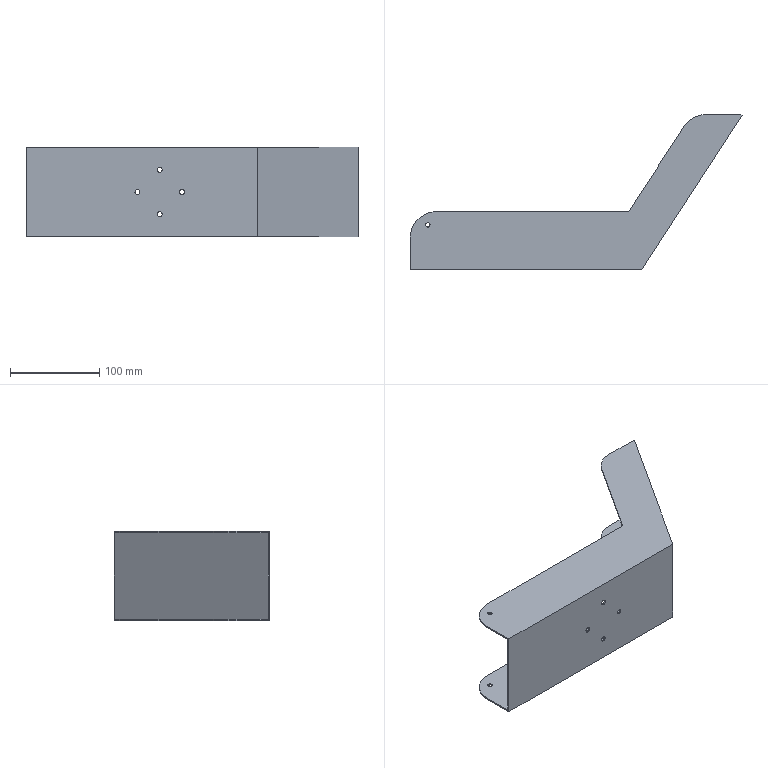Part | NX | 1 solid | 32 faces | box 372.47 x 174.005 x 100 mm | volume 140238 mm3 | plane 16 | cylinder 16 | commonest cylinder face diameters 5.5 x8 5 x4 60 x4
STEP:
#1=CARTESIAN_POINT('',(-165.999,174.005,50.));
#2=VERTEX_POINT('',#1);
#3=CARTESIAN_POINT('',(-127.288,174.005,50.));
#4=VERTEX_POINT('',#3);
#5=CARTESIAN_POINT('',(0.,174.005,50.));
#6=DIRECTION('',(1.,0.,0.));
#7=VECTOR('',#6,1000.);
#8=LINE('',#5,#7);
#9=EDGE_CURVE('',#2,#4,#8,.T.);
#10=ORIENTED_EDGE('',*,*,#9,.F.);
#11=CARTESIAN_POINT('',(-191.16,160.345,50.));
#12=VERTEX_POINT('',#11);
#13=CARTESIAN_POINT('',(-165.999,144.005,50.));
#14=DIRECTION('',(0.,0.,-1.));
#15=DIRECTION('',(-1.,0.,0.));
#16=AXIS2_PLACEMENT_3D('',#13,#14,#15);
#17=CIRCLE('',#16,30.);
#18=EDGE_CURVE('',#12,#2,#17,.T.);
#19=ORIENTED_EDGE('',*,*,#18,.F.);
#20=CARTESIAN_POINT('',(-253.077,65.,50.));
#21=VERTEX_POINT('',#20);
#22=CARTESIAN_POINT('',(-295.289,0.,50.));
#23=DIRECTION('',(0.5446,0.8387,0.));
#24=VECTOR('',#23,1000.);
#25=LINE('',#22,#24);
#26=EDGE_CURVE('',#21,#12,#25,.T.);
#27=ORIENTED_EDGE('',*,*,#26,.F.);
#28=CARTESIAN_POINT('',(-468.5,65.,50.));
#29=VERTEX_POINT('',#28);
#30=CARTESIAN_POINT('',(0.,65.,50.));
#31=DIRECTION('',(1.,0.,0.));
#32=VECTOR('',#31,1000.);
#33=LINE('',#30,#32);
#34=EDGE_CURVE('',#29,#21,#33,.T.);
#35=ORIENTED_EDGE('',*,*,#34,.F.);
#36=CARTESIAN_POINT('',(-498.5,35.,50.));
#37=VERTEX_POINT('',#36);
#38=CARTESIAN_POINT('',(-468.5,35.,50.));
#39=DIRECTION('',(0.,0.,1.));
#40=DIRECTION('',(1.,0.,0.));
#41=AXIS2_PLACEMENT_3D('',#38,#39,#40);
#42=CIRCLE('',#41,30.);
#43=EDGE_CURVE('',#29,#37,#42,.T.);
#44=ORIENTED_EDGE('',*,*,#43,.T.);
#45=CARTESIAN_POINT('',(-498.5,0.,50.));
#46=VERTEX_POINT('',#45);
#47=CARTESIAN_POINT('',(-498.5,0.,50.));
#48=DIRECTION('',(0.,-1.,0.));
#49=VECTOR('',#48,1000.);
#50=LINE('',#47,#49);
#51=EDGE_CURVE('',#37,#46,#50,.T.);
#52=ORIENTED_EDGE('',*,*,#51,.T.);
#53=CARTESIAN_POINT('',(-238.5,0.,50.));
#54=VERTEX_POINT('',#53);
#55=CARTESIAN_POINT('',(0.,0.,50.));
#56=DIRECTION('',(-1.,0.,0.));
#57=VECTOR('',#56,1000.);
#58=LINE('',#55,#57);
#59=EDGE_CURVE('',#54,#46,#58,.T.);
#60=ORIENTED_EDGE('',*,*,#59,.F.);
#61=CARTESIAN_POINT('',(-126.03,173.189,50.));
#62=VERTEX_POINT('',#61);
#63=CARTESIAN_POINT('',(-238.5,0.,50.));
#64=DIRECTION('',(-0.5446,-0.8387,0.));
#65=VECTOR('',#64,1000.);
#66=LINE('',#63,#65);
#67=EDGE_CURVE('',#62,#54,#66,.T.);
#68=ORIENTED_EDGE('',*,*,#67,.F.);
#69=CARTESIAN_POINT('',(0.,91.344,50.));
#70=DIRECTION('',(0.8387,-0.5446,0.));
#71=VECTOR('',#70,1000.);
#72=LINE('',#69,#71);
#73=EDGE_CURVE('',#4,#62,#72,.T.);
#74=ORIENTED_EDGE('',*,*,#73,.F.);
#75=EDGE_LOOP('',(#10,#19,#27,#35,#44,#52,#60,#68,#74));
#76=FACE_BOUND('',#75,.T.);
#77=CARTESIAN_POINT('',(-481.,50.,50.));
#78=VERTEX_POINT('',#77);
#79=CARTESIAN_POINT('',(-476.,50.,50.));
#80=VERTEX_POINT('',#79);
#81=CARTESIAN_POINT('',(-478.5,50.,50.));
#82=DIRECTION('',(0.,0.,1.));
#83=DIRECTION('',(1.,0.,0.));
#84=AXIS2_PLACEMENT_3D('',#81,#82,#83);
#85=CIRCLE('',#84,2.5);
#86=EDGE_CURVE('',#78,#80,#85,.T.);
#87=ORIENTED_EDGE('',*,*,#86,.F.);
#88=CARTESIAN_POINT('',(-478.5,50.,50.));
#89=DIRECTION('',(0.,0.,1.));
#90=DIRECTION('',(1.,0.,0.));
#91=AXIS2_PLACEMENT_3D('',#88,#89,#90);
#92=CIRCLE('',#91,2.5);
#93=EDGE_CURVE('',#80,#78,#92,.T.);
#94=ORIENTED_EDGE('',*,*,#93,.F.);
#95=EDGE_LOOP('',(#87,#94));
#96=FACE_BOUND('',#95,.T.);
#97=CARTESIAN_POINT('',(-221.19,55.831,50.));
#98=DIRECTION('',(0.,0.,1.));
#99=DIRECTION('',(1.,0.,0.));
#100=AXIS2_PLACEMENT_3D('',#97,#98,#99);
#101=PLANE('',#100);
#102=ADVANCED_FACE('',(#76,#96),#101,.T.);
#103=CARTESIAN_POINT('',(-468.5,65.,-48.5));
#104=VERTEX_POINT('',#103);
#105=CARTESIAN_POINT('',(-468.5,65.,-50.));
#106=VERTEX_POINT('',#105);
#107=CARTESIAN_POINT('',(-468.5,65.,0.));
#108=DIRECTION('',(0.,0.,-1.));
#109=VECTOR('',#108,1000.);
#110=LINE('',#107,#109);
#111=EDGE_CURVE('',#104,#106,#110,.T.);
#112=ORIENTED_EDGE('',*,*,#111,.F.);
#113=CARTESIAN_POINT('',(-253.077,65.,-48.5));
#114=VERTEX_POINT('',#113);
#115=CARTESIAN_POINT('',(0.,65.,-48.5));
#116=DIRECTION('',(1.,0.,0.));
#117=VECTOR('',#116,1000.);
#118=LINE('',#115,#117);
#119=EDGE_CURVE('',#104,#114,#118,.T.);
#120=ORIENTED_EDGE('',*,*,#119,.T.);
#121=CARTESIAN_POINT('',(-253.077,65.,-50.));
#122=VERTEX_POINT('',#121);
#123=CARTESIAN_POINT('',(-253.077,65.,0.));
#124=DIRECTION('',(0.,0.,-1.));
#125=VECTOR('',#124,1000.);
#126=LINE('',#123,#125);
#127=EDGE_CURVE('',#114,#122,#126,.T.);
#128=ORIENTED_EDGE('',*,*,#127,.T.);
#129=CARTESIAN_POINT('',(0.,65.,-50.));
#130=DIRECTION('',(1.,0.,0.));
#131=VECTOR('',#130,1000.);
#132=LINE('',#129,#131);
#133=EDGE_CURVE('',#106,#122,#132,.T.);
#134=ORIENTED_EDGE('',*,*,#133,.F.);
#135=EDGE_LOOP('',(#112,#120,#128,#134));
#136=FACE_BOUND('',#135,.T.);
#137=CARTESIAN_POINT('',(-249.25,65.,-59.25));
#138=DIRECTION('',(0.,-1.,0.));
#139=DIRECTION('',(0.,0.,-1.));
#140=AXIS2_PLACEMENT_3D('',#137,#138,#139);
#141=PLANE('',#140);
#142=ADVANCED_FACE('',(#136),#141,.F.);
#143=CARTESIAN_POINT('',(-239.314,1.5,-48.5));
#144=VERTEX_POINT('',#143);
#145=CARTESIAN_POINT('',(-127.288,174.005,-48.5));
#146=VERTEX_POINT('',#145);
#147=CARTESIAN_POINT('',(-240.289,0.,-48.5));
#148=DIRECTION('',(0.5446,0.8387,0.));
#149=VECTOR('',#148,1000.);
#150=LINE('',#147,#149);
#151=EDGE_CURVE('',#144,#146,#150,.T.);
#152=ORIENTED_EDGE('',*,*,#151,.T.);
#153=CARTESIAN_POINT('',(-165.999,174.005,-48.5));
#154=VERTEX_POINT('',#153);
#155=CARTESIAN_POINT('',(0.,174.005,-48.5));
#156=DIRECTION('',(-1.,0.,0.));
#157=VECTOR('',#156,1000.);
#158=LINE('',#155,#157);
#159=EDGE_CURVE('',#146,#154,#158,.T.);
#160=ORIENTED_EDGE('',*,*,#159,.T.);
#161=CARTESIAN_POINT('',(-191.16,160.345,-48.5));
#162=VERTEX_POINT('',#161);
#163=CARTESIAN_POINT('',(-165.999,144.005,-48.5));
#164=DIRECTION('',(0.,0.,1.));
#165=DIRECTION('',(1.,0.,0.));
#166=AXIS2_PLACEMENT_3D('',#163,#164,#165);
#167=CIRCLE('',#166,30.);
#168=EDGE_CURVE('',#154,#162,#167,.T.);
#169=ORIENTED_EDGE('',*,*,#168,.T.);
#170=CARTESIAN_POINT('',(-295.289,0.,-48.5));
#171=DIRECTION('',(-0.5446,-0.8387,0.));
#172=VECTOR('',#171,1000.);
#173=LINE('',#170,#172);
#174=EDGE_CURVE('',#162,#114,#173,.T.);
#175=ORIENTED_EDGE('',*,*,#174,.T.);
#176=ORIENTED_EDGE('',*,*,#119,.F.);
#177=CARTESIAN_POINT('',(-498.5,35.,-48.5));
#178=VERTEX_POINT('',#177);
#179=CARTESIAN_POINT('',(-468.5,35.,-48.5));
#180=DIRECTION('',(0.,0.,-1.));
#181=DIRECTION('',(-1.,0.,0.));
#182=AXIS2_PLACEMENT_3D('',#179,#180,#181);
#183=CIRCLE('',#182,30.);
#184=EDGE_CURVE('',#178,#104,#183,.T.);
#185=ORIENTED_EDGE('',*,*,#184,.F.);
#186=CARTESIAN_POINT('',(-498.5,1.5,-48.5));
#187=VERTEX_POINT('',#186);
#188=CARTESIAN_POINT('',(-498.5,0.,-48.5));
#189=DIRECTION('',(0.,1.,0.));
#190=VECTOR('',#189,1000.);
#191=LINE('',#188,#190);
#192=EDGE_CURVE('',#187,#178,#191,.T.);
#193=ORIENTED_EDGE('',*,*,#192,.F.);
#194=CARTESIAN_POINT('',(0.,1.5,-48.5));
#195=DIRECTION('',(1.,0.,0.));
#196=VECTOR('',#195,1000.);
#197=LINE('',#194,#196);
#198=EDGE_CURVE('',#187,#144,#197,.T.);
#199=ORIENTED_EDGE('',*,*,#198,.T.);
#200=EDGE_LOOP('',(#152,#160,#169,#175,#176,#185,#193,#199));
#201=FACE_BOUND('',#200,.T.);
#202=CARTESIAN_POINT('',(-476.,50.,-48.5));
#203=VERTEX_POINT('',#202);
#204=CARTESIAN_POINT('',(-481.,50.,-48.5));
#205=VERTEX_POINT('',#204);
#206=CARTESIAN_POINT('',(-478.5,50.,-48.5));
#207=DIRECTION('',(0.,0.,1.));
#208=DIRECTION('',(1.,0.,0.));
#209=AXIS2_PLACEMENT_3D('',#206,#207,#208);
#210=CIRCLE('',#209,2.5);
#211=EDGE_CURVE('',#203,#205,#210,.T.);
#212=ORIENTED_EDGE('',*,*,#211,.F.);
#213=CARTESIAN_POINT('',(-478.5,50.,-48.5));
#214=DIRECTION('',(0.,0.,1.));
#215=DIRECTION('',(1.,0.,0.));
#216=AXIS2_PLACEMENT_3D('',#213,#214,#215);
#217=CIRCLE('',#216,2.5);
#218=EDGE_CURVE('',#205,#203,#217,.T.);
#219=ORIENTED_EDGE('',*,*,#218,.F.);
#220=EDGE_LOOP('',(#212,#219));
#221=FACE_BOUND('',#220,.T.);
#222=CARTESIAN_POINT('',(-262.25,43.445,-48.5));
#223=DIRECTION('',(0.,0.,-1.));
#224=DIRECTION('',(0.,-1.,0.));
#225=AXIS2_PLACEMENT_3D('',#222,#223,#224);
#226=PLANE('',#225);
#227=ADVANCED_FACE('',(#201,#221),#226,.F.);
#228=CARTESIAN_POINT('',(-320.75,0.,0.));
#229=VERTEX_POINT('',#228);
#230=CARTESIAN_POINT('',(-326.25,0.,0.));
#231=VERTEX_POINT('',#230);
#232=CARTESIAN_POINT('',(-323.5,0.,0.));
#233=DIRECTION('',(0.,-1.,0.));
#234=DIRECTION('',(-1.,0.,0.));
#235=AXIS2_PLACEMENT_3D('',#232,#233,#234);
#236=CIRCLE('',#235,2.75);
#237=EDGE_CURVE('',#229,#231,#236,.T.);
#238=ORIENTED_EDGE('',*,*,#237,.T.);
#239=CARTESIAN_POINT('',(-326.25,1.5,0.));
#240=VERTEX_POINT('',#239);
#241=CARTESIAN_POINT('',(-326.25,1.5,0.));
#242=DIRECTION('',(0.,-1.,0.));
#243=VECTOR('',#242,1000.);
#244=LINE('',#241,#243);
#245=EDGE_CURVE('',#231,#240,#244,.F.);
#246=ORIENTED_EDGE('',*,*,#245,.T.);
#247=CARTESIAN_POINT('',(-320.75,1.5,0.));
#248=VERTEX_POINT('',#247);
#249=CARTESIAN_POINT('',(-323.5,1.5,0.));
#250=DIRECTION('',(0.,1.,0.));
#251=DIRECTION('',(1.,0.,0.));
#252=AXIS2_PLACEMENT_3D('',#249,#250,#251);
#253=CIRCLE('',#252,2.75);
#254=EDGE_CURVE('',#240,#248,#253,.T.);
#255=ORIENTED_EDGE('',*,*,#254,.T.);
#256=CARTESIAN_POINT('',(-320.75,1.5,0.));
#257=DIRECTION('',(0.,-1.,0.));
#258=VECTOR('',#257,1000.);
#259=LINE('',#256,#258);
#260=EDGE_CURVE('',#229,#248,#259,.F.);
#261=ORIENTED_EDGE('',*,*,#260,.F.);
#262=EDGE_LOOP('',(#238,#246,#255,#261));
#263=FACE_BOUND('',#262,.T.);
#264=CARTESIAN_POINT('',(-323.5,1.5,0.));
#265=DIRECTION('',(0.,-1.,0.));
#266=DIRECTION('',(1.,0.,0.));
#267=AXIS2_PLACEMENT_3D('',#264,#265,#266);
#268=CYLINDRICAL_SURFACE('',#267,2.75);
#269=ADVANCED_FACE('',(#263),#268,.F.);
#270=CARTESIAN_POINT('',(-351.25,0.,-25.));
#271=VERTEX_POINT('',#270);
#272=CARTESIAN_POINT('',(-345.75,0.,-25.));
#273=VERTEX_POINT('',#272);
#274=CARTESIAN_POINT('',(-348.5,0.,-25.));
#275=DIRECTION('',(0.,-1.,0.));
#276=DIRECTION('',(-1.,0.,0.));
#277=AXIS2_PLACEMENT_3D('',#274,#275,#276);
#278=CIRCLE('',#277,2.75);
#279=EDGE_CURVE('',#271,#273,#278,.T.);
#280=ORIENTED_EDGE('',*,*,#279,.T.);
#281=CARTESIAN_POINT('',(-345.75,1.5,-25.));
#282=VERTEX_POINT('',#281);
#283=CARTESIAN_POINT('',(-345.75,1.5,-25.));
#284=DIRECTION('',(0.,-1.,0.));
#285=VECTOR('',#284,1000.);
#286=LINE('',#283,#285);
#287=EDGE_CURVE('',#282,#273,#286,.T.);
#288=ORIENTED_EDGE('',*,*,#287,.F.);
#289=CARTESIAN_POINT('',(-351.25,1.5,-25.));
#290=VERTEX_POINT('',#289);
#291=CARTESIAN_POINT('',(-348.5,1.5,-25.));
#292=DIRECTION('',(0.,1.,0.));
#293=DIRECTION('',(1.,0.,0.));
#294=AXIS2_PLACEMENT_3D('',#291,#292,#293);
#295=CIRCLE('',#294,2.75);
#296=EDGE_CURVE('',#282,#290,#295,.T.);
#297=ORIENTED_EDGE('',*,*,#296,.T.);
#298=CARTESIAN_POINT('',(-351.25,1.5,-25.));
#299=DIRECTION('',(0.,-1.,0.));
#300=VECTOR('',#299,1000.);
#301=LINE('',#298,#300);
#302=EDGE_CURVE('',#290,#271,#301,.T.);
#303=ORIENTED_EDGE('',*,*,#302,.T.);
#304=EDGE_LOOP('',(#280,#288,#297,#303));
#305=FACE_BOUND('',#304,.T.);
#306=CARTESIAN_POINT('',(-348.5,1.5,-25.));
#307=DIRECTION('',(0.,-1.,0.));
#308=DIRECTION('',(1.,0.,0.));
#309=AXIS2_PLACEMENT_3D('',#306,#307,#308);
#310=CYLINDRICAL_SURFACE('',#309,2.75);
#311=ADVANCED_FACE('',(#305),#310,.F.);
#312=CARTESIAN_POINT('',(-468.5,65.,48.5));
#313=VERTEX_POINT('',#312);
#314=CARTESIAN_POINT('',(-468.5,65.,60.003));
#315=DIRECTION('',(0.,0.,-1.));
#316=VECTOR('',#315,1000.);
#317=LINE('',#314,#316);
#318=EDGE_CURVE('',#29,#313,#317,.T.);
#319=ORIENTED_EDGE('',*,*,#318,.F.);
#320=ORIENTED_EDGE('',*,*,#34,.T.);
#321=CARTESIAN_POINT('',(-253.077,65.,48.5));
#322=VERTEX_POINT('',#321);
#323=CARTESIAN_POINT('',(-253.077,65.,0.));
#324=DIRECTION('',(0.,0.,1.));
#325=VECTOR('',#324,1000.);
#326=LINE('',#323,#325);
#327=EDGE_CURVE('',#322,#21,#326,.T.);
#328=ORIENTED_EDGE('',*,*,#327,.F.);
#329=CARTESIAN_POINT('',(0.,65.,48.5));
#330=DIRECTION('',(1.,0.,0.));
#331=VECTOR('',#330,1000.);
#332=LINE('',#329,#331);
#333=EDGE_CURVE('',#313,#322,#332,.T.);
#334=ORIENTED_EDGE('',*,*,#333,.F.);
#335=EDGE_LOOP('',(#319,#320,#328,#334));
#336=FACE_BOUND('',#335,.T.);
#337=CARTESIAN_POINT('',(-249.25,65.,59.25));
#338=DIRECTION('',(0.,1.,0.));
#339=DIRECTION('',(1.,0.,0.));
#340=AXIS2_PLACEMENT_3D('',#337,#338,#339);
#341=PLANE('',#340);
#342=ADVANCED_FACE('',(#336),#341,.T.);
#343=ORIENTED_EDGE('',*,*,#86,.T.);
#344=CARTESIAN_POINT('',(-476.,50.,48.5));
#345=VERTEX_POINT('',#344);
#346=CARTESIAN_POINT('',(-476.,50.,72.));
#347=DIRECTION('',(0.,0.,1.));
#348=VECTOR('',#347,1000.);
#349=LINE('',#346,#348);
#350=EDGE_CURVE('',#345,#80,#349,.T.);
#351=ORIENTED_EDGE('',*,*,#350,.F.);
#352=CARTESIAN_POINT('',(-481.,50.,48.5));
#353=VERTEX_POINT('',#352);
#354=CARTESIAN_POINT('',(-478.5,50.,48.5));
#355=DIRECTION('',(0.,0.,1.));
#356=DIRECTION('',(1.,0.,0.));
#357=AXIS2_PLACEMENT_3D('',#354,#355,#356);
#358=CIRCLE('',#357,2.5);
#359=EDGE_CURVE('',#353,#345,#358,.T.);
#360=ORIENTED_EDGE('',*,*,#359,.F.);
#361=CARTESIAN_POINT('',(-481.,50.,72.));
#362=DIRECTION('',(0.,0.,1.));
#363=VECTOR('',#362,1000.);
#364=LINE('',#361,#363);
#365=EDGE_CURVE('',#353,#78,#364,.T.);
#366=ORIENTED_EDGE('',*,*,#365,.T.);
#367=EDGE_LOOP('',(#343,#351,#360,#366));
#368=FACE_BOUND('',#367,.T.);
#369=CARTESIAN_POINT('',(-478.5,50.,72.));
#370=DIRECTION('',(0.,0.,1.));
#371=DIRECTION('',(1.,0.,0.));
#372=AXIS2_PLACEMENT_3D('',#369,#370,#371);
#373=CYLINDRICAL_SURFACE('',#372,2.5);
#374=ADVANCED_FACE('',(#368),#373,.F.);
#375=CARTESIAN_POINT('',(-239.314,1.5,48.5));
#376=VERTEX_POINT('',#375);
#377=CARTESIAN_POINT('',(-239.314,1.5,0.));
#378=DIRECTION('',(0.,0.,1.));
#379=VECTOR('',#378,1000.);
#380=LINE('',#377,#379);
#381=EDGE_CURVE('',#144,#376,#380,.T.);
#382=ORIENTED_EDGE('',*,*,#381,.F.);
#383=ORIENTED_EDGE('',*,*,#198,.F.);
#384=CARTESIAN_POINT('',(-498.5,1.5,48.5));
#385=VERTEX_POINT('',#384);
#386=CARTESIAN_POINT('',(-498.5,1.5,0.));
#387=DIRECTION('',(0.,0.,1.));
#388=VECTOR('',#387,1000.);
#389=LINE('',#386,#388);
#390=EDGE_CURVE('',#187,#385,#389,.T.);
#391=ORIENTED_EDGE('',*,*,#390,.T.);
#392=CARTESIAN_POINT('',(0.,1.5,48.5));
#393=DIRECTION('',(-1.,0.,0.));
#394=VECTOR('',#393,1000.);
#395=LINE('',#392,#394);
#396=EDGE_CURVE('',#376,#385,#395,.T.);
#397=ORIENTED_EDGE('',*,*,#396,.F.);
#398=EDGE_LOOP('',(#382,#383,#391,#397));
#399=FACE_BOUND('',#398,.T.);
#400=CARTESIAN_POINT('',(-370.75,1.5,0.));
#401=VERTEX_POINT('',#400);
#402=CARTESIAN_POINT('',(-376.25,1.5,0.));
#403=VERTEX_POINT('',#402);
#404=CARTESIAN_POINT('',(-373.5,1.5,0.));
#405=DIRECTION('',(0.,1.,0.));
#406=DIRECTION('',(1.,0.,0.));
#407=AXIS2_PLACEMENT_3D('',#404,#405,#406);
#408=CIRCLE('',#407,2.75);
#409=EDGE_CURVE('',#401,#403,#408,.T.);
#410=ORIENTED_EDGE('',*,*,#409,.F.);
#411=CARTESIAN_POINT('',(-373.5,1.5,0.));
#412=DIRECTION('',(0.,1.,0.));
#413=DIRECTION('',(1.,0.,0.));
#414=AXIS2_PLACEMENT_3D('',#411,#412,#413);
#415=CIRCLE('',#414,2.75);
#416=EDGE_CURVE('',#403,#401,#415,.T.);
#417=ORIENTED_EDGE('',*,*,#416,.F.);
#418=EDGE_LOOP('',(#410,#417));
#419=FACE_BOUND('',#418,.T.);
#420=CARTESIAN_POINT('',(-345.75,1.5,25.));
#421=VERTEX_POINT('',#420);
#422=CARTESIAN_POINT('',(-351.25,1.5,25.));
#423=VERTEX_POINT('',#422);
#424=CARTESIAN_POINT('',(-348.5,1.5,25.));
#425=DIRECTION('',(0.,1.,0.));
#426=DIRECTION('',(1.,0.,0.));
#427=AXIS2_PLACEMENT_3D('',#424,#425,#426);
#428=CIRCLE('',#427,2.75);
#429=EDGE_CURVE('',#421,#423,#428,.T.);
#430=ORIENTED_EDGE('',*,*,#429,.F.);
#431=CARTESIAN_POINT('',(-348.5,1.5,25.));
#432=DIRECTION('',(0.,1.,0.));
#433=DIRECTION('',(1.,0.,0.));
#434=AXIS2_PLACEMENT_3D('',#431,#432,#433);
#435=CIRCLE('',#434,2.75);
#436=EDGE_CURVE('',#423,#421,#435,.T.);
#437=ORIENTED_EDGE('',*,*,#436,.F.);
#438=EDGE_LOOP('',(#430,#437));
#439=FACE_BOUND('',#438,.T.);
#440=CARTESIAN_POINT('',(-348.5,1.5,-25.));
#441=DIRECTION('',(0.,1.,0.));
#442=DIRECTION('',(1.,0.,0.));
#443=AXIS2_PLACEMENT_3D('',#440,#441,#442);
#444=CIRCLE('',#443,2.75);
#445=EDGE_CURVE('',#290,#282,#444,.T.);
#446=ORIENTED_EDGE('',*,*,#445,.F.);
#447=ORIENTED_EDGE('',*,*,#296,.F.);
#448=EDGE_LOOP('',(#446,#447));
#449=FACE_BOUND('',#448,.T.);
#450=CARTESIAN_POINT('',(-323.5,1.5,0.));
#451=DIRECTION('',(0.,1.,0.));
#452=DIRECTION('',(1.,0.,0.));
#453=AXIS2_PLACEMENT_3D('',#450,#451,#452);
#454=CIRCLE('',#453,2.75);
#455=EDGE_CURVE('',#248,#240,#454,.T.);
#456=ORIENTED_EDGE('',*,*,#455,.F.);
#457=ORIENTED_EDGE('',*,*,#254,.F.);
#458=EDGE_LOOP('',(#456,#457));
#459=FACE_BOUND('',#458,.T.);
#460=CARTESIAN_POINT('',(0.,1.5,60.));
#461=DIRECTION('',(0.,-1.,0.));
#462=DIRECTION('',(0.,0.,-1.));
#463=AXIS2_PLACEMENT_3D('',#460,#461,#462);
#464=PLANE('',#463);
#465=ADVANCED_FACE('',(#399,#419,#439,#449,#459),#464,.F.);
#466=CARTESIAN_POINT('',(-191.16,160.345,48.5));
#467=VERTEX_POINT('',#466);
#468=CARTESIAN_POINT('',(-191.16,160.345,0.));
#469=DIRECTION('',(0.,0.,-1.));
#470=VECTOR('',#469,1000.);
#471=LINE('',#468,#470);
#472=EDGE_CURVE('',#12,#467,#471,.T.);
#473=ORIENTED_EDGE('',*,*,#472,.T.);
#474=CARTESIAN_POINT('',(-295.289,0.,48.5));
#475=DIRECTION('',(0.5446,0.8387,0.));
#476=VECTOR('',#475,1000.);
#477=LINE('',#474,#476);
#478=EDGE_CURVE('',#322,#467,#477,.T.);
#479=ORIENTED_EDGE('',*,*,#478,.F.);
#480=ORIENTED_EDGE('',*,*,#327,.T.);
#481=ORIENTED_EDGE('',*,*,#26,.T.);
#482=EDGE_LOOP('',(#473,#479,#480,#481));
#483=FACE_BOUND('',#482,.T.);
#484=CARTESIAN_POINT('',(-182.288,174.005,60.));
#485=DIRECTION('',(-0.8387,0.5446,0.));
#486=DIRECTION('',(0.,0.,1.));
#487=AXIS2_PLACEMENT_3D('',#484,#485,#486);
#488=PLANE('',#487);
#489=ADVANCED_FACE('',(#483),#488,.T.);
#490=ORIENTED_EDGE('',*,*,#59,.T.);
#491=CARTESIAN_POINT('',(-498.5,0.,-50.));
#492=VERTEX_POINT('',#491);
#493=CARTESIAN_POINT('',(-498.5,0.,0.));
#494=DIRECTION('',(0.,0.,1.));
#495=VECTOR('',#494,1000.);
#496=LINE('',#493,#495);
#497=EDGE_CURVE('',#492,#46,#496,.T.);
#498=ORIENTED_EDGE('',*,*,#497,.F.);
#499=CARTESIAN_POINT('',(-238.5,0.,-50.));
#500=VERTEX_POINT('',#499);
#501=CARTESIAN_POINT('',(0.,0.,-50.));
#502=DIRECTION('',(1.,0.,0.));
#503=VECTOR('',#502,1000.);
#504=LINE('',#501,#503);
#505=EDGE_CURVE('',#492,#500,#504,.T.);
#506=ORIENTED_EDGE('',*,*,#505,.T.);
#507=CARTESIAN_POINT('',(-238.5,0.,0.));
#508=DIRECTION('',(0.,0.,-1.));
#509=VECTOR('',#508,1000.);
#510=LINE('',#507,#509);
#511=EDGE_CURVE('',#54,#500,#510,.T.);
#512=ORIENTED_EDGE('',*,*,#511,.F.);
#513=EDGE_LOOP('',(#490,#498,#506,#512));
#514=FACE_BOUND('',#513,.T.);
#515=CARTESIAN_POINT('',(-376.25,0.,0.));
#516=VERTEX_POINT('',#515);
#517=CARTESIAN_POINT('',(-370.75,0.,0.));
#518=VERTEX_POINT('',#517);
#519=CARTESIAN_POINT('',(-373.5,0.,0.));
#520=DIRECTION('',(0.,-1.,0.));
#521=DIRECTION('',(-1.,0.,0.));
#522=AXIS2_PLACEMENT_3D('',#519,#520,#521);
#523=CIRCLE('',#522,2.75);
#524=EDGE_CURVE('',#516,#518,#523,.T.);
#525=ORIENTED_EDGE('',*,*,#524,.F.);
#526=CARTESIAN_POINT('',(-373.5,0.,0.));
#527=DIRECTION('',(0.,-1.,0.));
#528=DIRECTION('',(-1.,0.,0.));
#529=AXIS2_PLACEMENT_3D('',#526,#527,#528);
#530=CIRCLE('',#529,2.75);
#531=EDGE_CURVE('',#518,#516,#530,.T.);
#532=ORIENTED_EDGE('',*,*,#531,.F.);
#533=EDGE_LOOP('',(#525,#532));
#534=FACE_BOUND('',#533,.T.);
#535=CARTESIAN_POINT('',(-345.75,0.,25.));
#536=VERTEX_POINT('',#535);
#537=CARTESIAN_POINT('',(-351.25,0.,25.));
#538=VERTEX_POINT('',#537);
#539=CARTESIAN_POINT('',(-348.5,0.,25.));
#540=DIRECTION('',(0.,-1.,0.));
#541=DIRECTION('',(-1.,0.,0.));
#542=AXIS2_PLACEMENT_3D('',#539,#540,#541);
#543=CIRCLE('',#542,2.75);
#544=EDGE_CURVE('',#536,#538,#543,.T.);
#545=ORIENTED_EDGE('',*,*,#544,.F.);
#546=CARTESIAN_POINT('',(-348.5,0.,25.));
#547=DIRECTION('',(0.,-1.,0.));
#548=DIRECTION('',(-1.,0.,0.));
#549=AXIS2_PLACEMENT_3D('',#546,#547,#548);
#550=CIRCLE('',#549,2.75);
#551=EDGE_CURVE('',#538,#536,#550,.T.);
#552=ORIENTED_EDGE('',*,*,#551,.F.);
#553=EDGE_LOOP('',(#545,#552));
#554=FACE_BOUND('',#553,.T.);
#555=ORIENTED_EDGE('',*,*,#279,.F.);
#556=CARTESIAN_POINT('',(-348.5,0.,-25.));
#557=DIRECTION('',(0.,-1.,0.));
#558=DIRECTION('',(-1.,0.,0.));
#559=AXIS2_PLACEMENT_3D('',#556,#557,#558);
#560=CIRCLE('',#559,2.75);
#561=EDGE_CURVE('',#273,#271,#560,.T.);
#562=ORIENTED_EDGE('',*,*,#561,.F.);
#563=EDGE_LOOP('',(#555,#562));
#564=FACE_BOUND('',#563,.T.);
#565=ORIENTED_EDGE('',*,*,#237,.F.);
#566=CARTESIAN_POINT('',(-323.5,0.,0.));
#567=DIRECTION('',(0.,-1.,0.));
#568=DIRECTION('',(-1.,0.,0.));
#569=AXIS2_PLACEMENT_3D('',#566,#567,#568);
#570=CIRCLE('',#569,2.75);
#571=EDGE_CURVE('',#231,#229,#570,.T.);
#572=ORIENTED_EDGE('',*,*,#571,.F.);
#573=EDGE_LOOP('',(#565,#572));
#574=FACE_BOUND('',#573,.T.);
#575=CARTESIAN_POINT('',(0.,0.,60.));
#576=DIRECTION('',(0.,-1.,0.));
#577=DIRECTION('',(0.,0.,-1.));
#578=AXIS2_PLACEMENT_3D('',#575,#576,#577);
#579=PLANE('',#578);
#580=ADVANCED_FACE('',(#514,#534,#554,#564,#574),#579,.T.);
#581=ORIENTED_EDGE('',*,*,#211,.T.);
#582=CARTESIAN_POINT('',(-481.,50.,-50.));
#583=VERTEX_POINT('',#582);
#584=CARTESIAN_POINT('',(-481.,50.,72.));
#585=DIRECTION('',(0.,0.,1.));
#586=VECTOR('',#585,1000.);
#587=LINE('',#584,#586);
#588=EDGE_CURVE('',#583,#205,#587,.T.);
#589=ORIENTED_EDGE('',*,*,#588,.F.);
#590=CARTESIAN_POINT('',(-476.,50.,-50.));
#591=VERTEX_POINT('',#590);
#592=CARTESIAN_POINT('',(-478.5,50.,-50.));
#593=DIRECTION('',(0.,0.,1.));
#594=DIRECTION('',(1.,0.,0.));
#595=AXIS2_PLACEMENT_3D('',#592,#593,#594);
#596=CIRCLE('',#595,2.5);
#597=EDGE_CURVE('',#591,#583,#596,.T.);
#598=ORIENTED_EDGE('',*,*,#597,.F.);
#599=CARTESIAN_POINT('',(-476.,50.,72.));
#600=DIRECTION('',(0.,0.,1.));
#601=VECTOR('',#600,1000.);
#602=LINE('',#599,#601);
#603=EDGE_CURVE('',#591,#203,#602,.T.);
#604=ORIENTED_EDGE('',*,*,#603,.T.);
#605=EDGE_LOOP('',(#581,#589,#598,#604));
#606=FACE_BOUND('',#605,.T.);
#607=CARTESIAN_POINT('',(-478.5,50.,72.));
#608=DIRECTION('',(0.,0.,1.));
#609=DIRECTION('',(1.,0.,0.));
#610=AXIS2_PLACEMENT_3D('',#607,#608,#609);
#611=CYLINDRICAL_SURFACE('',#610,2.5);
#612=ADVANCED_FACE('',(#606),#611,.F.);
#613=CARTESIAN_POINT('',(-498.5,35.,-50.));
#614=VERTEX_POINT('',#613);
#615=CARTESIAN_POINT('',(-498.5,35.,0.));
#616=DIRECTION('',(0.,0.,-1.));
#617=VECTOR('',#616,1000.);
#618=LINE('',#615,#617);
#619=EDGE_CURVE('',#178,#614,#618,.T.);
#620=ORIENTED_EDGE('',*,*,#619,.F.);
#621=ORIENTED_EDGE('',*,*,#184,.T.);
#622=ORIENTED_EDGE('',*,*,#111,.T.);
#623=CARTESIAN_POINT('',(-468.5,35.,-50.));
#624=DIRECTION('',(0.,0.,-1.));
#625=DIRECTION('',(-1.,0.,0.));
#626=AXIS2_PLACEMENT_3D('',#623,#624,#625);
#627=CIRCLE('',#626,30.);
#628=EDGE_CURVE('',#614,#106,#627,.T.);
#629=ORIENTED_EDGE('',*,*,#628,.F.);
#630=EDGE_LOOP('',(#620,#621,#622,#629));
#631=FACE_BOUND('',#630,.T.);
#632=CARTESIAN_POINT('',(-468.5,35.,0.));
#633=DIRECTION('',(0.,0.,-1.));
#634=DIRECTION('',(-1.,0.,0.));
#635=AXIS2_PLACEMENT_3D('',#632,#633,#634);
#636=CYLINDRICAL_SURFACE('',#635,30.);
#637=ADVANCED_FACE('',(#631),#636,.T.);
#638=ORIENTED_EDGE('',*,*,#429,.T.);
#639=CARTESIAN_POINT('',(-351.25,1.5,25.));
#640=DIRECTION('',(0.,-1.,0.));
#641=VECTOR('',#640,1000.);
#642=LINE('',#639,#641);
#643=EDGE_CURVE('',#538,#423,#642,.F.);
#644=ORIENTED_EDGE('',*,*,#643,.F.);
#645=ORIENTED_EDGE('',*,*,#551,.T.);
#646=CARTESIAN_POINT('',(-345.75,1.5,25.));
#647=DIRECTION('',(0.,-1.,0.));
#648=VECTOR('',#647,1000.);
#649=LINE('',#646,#648);
#650=EDGE_CURVE('',#536,#421,#649,.F.);
#651=ORIENTED_EDGE('',*,*,#650,.T.);
#652=EDGE_LOOP('',(#638,#644,#645,#651));
#653=FACE_BOUND('',#652,.T.);
#654=CARTESIAN_POINT('',(-348.5,1.5,25.));
#655=DIRECTION('',(0.,-1.,0.));
#656=DIRECTION('',(1.,0.,0.));
#657=AXIS2_PLACEMENT_3D('',#654,#655,#656);
#658=CYLINDRICAL_SURFACE('',#657,2.75);
#659=ADVANCED_FACE('',(#653),#658,.F.);
#660=CARTESIAN_POINT('',(-191.16,160.345,-50.));
#661=VERTEX_POINT('',#660);
#662=CARTESIAN_POINT('',(-191.16,160.345,0.));
#663=DIRECTION('',(0.,0.,1.));
#664=VECTOR('',#663,1000.);
#665=LINE('',#662,#664);
#666=EDGE_CURVE('',#661,#162,#665,.T.);
#667=ORIENTED_EDGE('',*,*,#666,.F.);
#668=CARTESIAN_POINT('',(-295.289,0.,-50.));
#669=DIRECTION('',(-0.5446,-0.8387,0.));
#670=VECTOR('',#669,1000.);
#671=LINE('',#668,#670);
#672=EDGE_CURVE('',#661,#122,#671,.T.);
#673=ORIENTED_EDGE('',*,*,#672,.T.);
#674=ORIENTED_EDGE('',*,*,#127,.F.);
#675=ORIENTED_EDGE('',*,*,#174,.F.);
#676=EDGE_LOOP('',(#667,#673,#674,#675));
#677=FACE_BOUND('',#676,.T.);
#678=CARTESIAN_POINT('',(-253.077,65.,-60.));
#679=DIRECTION('',(-0.8387,0.5446,0.));
#680=DIRECTION('',(0.,0.,1.));
#681=AXIS2_PLACEMENT_3D('',#678,#679,#680);
#682=PLANE('',#681);
#683=ADVANCED_FACE('',(#677),#682,.T.);
#684=ORIENTED_EDGE('',*,*,#318,.T.);
#685=CARTESIAN_POINT('',(-498.5,35.,48.5));
#686=VERTEX_POINT('',#685);
#687=CARTESIAN_POINT('',(-468.5,35.,48.5));
#688=DIRECTION('',(0.,0.,1.));
#689=DIRECTION('',(1.,0.,0.));
#690=AXIS2_PLACEMENT_3D('',#687,#688,#689);
#691=CIRCLE('',#690,30.);
#692=EDGE_CURVE('',#313,#686,#691,.T.);
#693=ORIENTED_EDGE('',*,*,#692,.T.);
#694=CARTESIAN_POINT('',(-498.5,35.,0.));
#695=DIRECTION('',(0.,0.,1.));
#696=VECTOR('',#695,1000.);
#697=LINE('',#694,#696);
#698=EDGE_CURVE('',#686,#37,#697,.T.);
#699=ORIENTED_EDGE('',*,*,#698,.T.);
#700=ORIENTED_EDGE('',*,*,#43,.F.);
#701=EDGE_LOOP('',(#684,#693,#699,#700));
#702=FACE_BOUND('',#701,.T.);
#703=CARTESIAN_POINT('',(-468.5,35.,0.));
#704=DIRECTION('',(0.,0.,1.));
#705=DIRECTION('',(1.,0.,0.));
#706=AXIS2_PLACEMENT_3D('',#703,#704,#705);
#707=CYLINDRICAL_SURFACE('',#706,30.);
#708=ADVANCED_FACE('',(#702),#707,.T.);
#709=CARTESIAN_POINT('',(-165.999,174.005,48.5));
#710=VERTEX_POINT('',#709);
#711=CARTESIAN_POINT('',(-127.288,174.005,48.5));
#712=VERTEX_POINT('',#711);
#713=CARTESIAN_POINT('',(0.,174.005,48.5));
#714=DIRECTION('',(1.,0.,0.));
#715=VECTOR('',#714,1000.);
#716=LINE('',#713,#715);
#717=EDGE_CURVE('',#710,#712,#716,.T.);
#718=ORIENTED_EDGE('',*,*,#717,.F.);
#719=CARTESIAN_POINT('',(-165.999,174.005,0.));
#720=DIRECTION('',(0.,0.,-1.));
#721=VECTOR('',#720,1000.);
#722=LINE('',#719,#721);
#723=EDGE_CURVE('',#2,#710,#722,.T.);
#724=ORIENTED_EDGE('',*,*,#723,.F.);
#725=ORIENTED_EDGE('',*,*,#9,.T.);
#726=CARTESIAN_POINT('',(-127.288,174.005,0.));
#727=DIRECTION('',(0.,0.,1.));
#728=VECTOR('',#727,1000.);
#729=LINE('',#726,#728);
#730=EDGE_CURVE('',#712,#4,#729,.T.);
#731=ORIENTED_EDGE('',*,*,#730,.F.);
#732=EDGE_LOOP('',(#718,#724,#725,#731));
#733=FACE_BOUND('',#732,.T.);
#734=CARTESIAN_POINT('',(-127.288,174.005,60.));
#735=DIRECTION('',(0.,1.,0.));
#736=DIRECTION('',(1.,0.,0.));
#737=AXIS2_PLACEMENT_3D('',#734,#735,#736);
#738=PLANE('',#737);
#739=ADVANCED_FACE('',(#733),#738,.T.);
#740=ORIENTED_EDGE('',*,*,#409,.T.);
#741=CARTESIAN_POINT('',(-376.25,1.5,0.));
#742=DIRECTION('',(0.,-1.,0.));
#743=VECTOR('',#742,1000.);
#744=LINE('',#741,#743);
#745=EDGE_CURVE('',#403,#516,#744,.T.);
#746=ORIENTED_EDGE('',*,*,#745,.T.);
#747=ORIENTED_EDGE('',*,*,#524,.T.);
#748=CARTESIAN_POINT('',(-370.75,1.5,0.));
#749=DIRECTION('',(0.,-1.,0.));
#750=VECTOR('',#749,1000.);
#751=LINE('',#748,#750);
#752=EDGE_CURVE('',#401,#518,#751,.T.);
#753=ORIENTED_EDGE('',*,*,#752,.F.);
#754=EDGE_LOOP('',(#740,#746,#747,#753));
#755=FACE_BOUND('',#754,.T.);
#756=CARTESIAN_POINT('',(-373.5,1.5,0.));
#757=DIRECTION('',(0.,-1.,0.));
#758=DIRECTION('',(1.,0.,0.));
#759=AXIS2_PLACEMENT_3D('',#756,#757,#758);
#760=CYLINDRICAL_SURFACE('',#759,2.75);
#761=ADVANCED_FACE('',(#755),#760,.F.);
#762=CARTESIAN_POINT('',(-127.288,174.005,60.));
#763=DIRECTION('',(0.,0.,-1.));
#764=VECTOR('',#763,1000.);
#765=LINE('',#762,#764);
#766=EDGE_CURVE('',#712,#146,#765,.T.);
#767=ORIENTED_EDGE('',*,*,#766,.F.);
#768=ORIENTED_EDGE('',*,*,#730,.T.);
#769=ORIENTED_EDGE('',*,*,#73,.T.);
#770=CARTESIAN_POINT('',(-126.03,173.189,-50.));
#771=VERTEX_POINT('',#770);
#772=CARTESIAN_POINT('',(-126.03,173.189,0.));
#773=DIRECTION('',(0.,0.,-1.));
#774=VECTOR('',#773,1000.);
#775=LINE('',#772,#774);
#776=EDGE_CURVE('',#62,#771,#775,.T.);
#777=ORIENTED_EDGE('',*,*,#776,.T.);
#778=CARTESIAN_POINT('',(-127.288,174.005,-50.));
#779=VERTEX_POINT('',#778);
#780=CARTESIAN_POINT('',(0.,91.344,-50.));
#781=DIRECTION('',(-0.8387,0.5446,0.));
#782=VECTOR('',#781,1000.);
#783=LINE('',#780,#782);
#784=EDGE_CURVE('',#771,#779,#783,.T.);
#785=ORIENTED_EDGE('',*,*,#784,.T.);
#786=CARTESIAN_POINT('',(-127.288,174.005,0.));
#787=DIRECTION('',(0.,0.,-1.));
#788=VECTOR('',#787,1000.);
#789=LINE('',#786,#788);
#790=EDGE_CURVE('',#146,#779,#789,.T.);
#791=ORIENTED_EDGE('',*,*,#790,.F.);
#792=EDGE_LOOP('',(#767,#768,#769,#777,#785,#791));
#793=FACE_BOUND('',#792,.T.);
#794=CARTESIAN_POINT('',(-126.03,173.189,-60.));
#795=DIRECTION('',(0.5446,0.8387,0.));
#796=DIRECTION('',(0.,0.,-1.));
#797=AXIS2_PLACEMENT_3D('',#794,#795,#796);
#798=PLANE('',#797);
#799=ADVANCED_FACE('',(#793),#798,.T.);
#800=ORIENTED_EDGE('',*,*,#67,.T.);
#801=ORIENTED_EDGE('',*,*,#511,.T.);
#802=CARTESIAN_POINT('',(-238.5,0.,-50.));
#803=DIRECTION('',(0.5446,0.8387,0.));
#804=VECTOR('',#803,1000.);
#805=LINE('',#802,#804);
#806=EDGE_CURVE('',#500,#771,#805,.T.);
#807=ORIENTED_EDGE('',*,*,#806,.T.);
#808=ORIENTED_EDGE('',*,*,#776,.F.);
#809=EDGE_LOOP('',(#800,#801,#807,#808));
#810=FACE_BOUND('',#809,.T.);
#811=CARTESIAN_POINT('',(-238.268,0.3574,57.296));
#812=DIRECTION('',(0.8387,-0.5446,0.));
#813=DIRECTION('',(0.,0.,-1.));
#814=AXIS2_PLACEMENT_3D('',#811,#812,#813);
#815=PLANE('',#814);
#816=ADVANCED_FACE('',(#810),#815,.T.);
#817=CARTESIAN_POINT('',(-240.289,0.,48.5));
#818=DIRECTION('',(-0.5446,-0.8387,0.));
#819=VECTOR('',#818,1000.);
#820=LINE('',#817,#819);
#821=EDGE_CURVE('',#712,#376,#820,.T.);
#822=ORIENTED_EDGE('',*,*,#821,.T.);
#823=ORIENTED_EDGE('',*,*,#396,.T.);
#824=CARTESIAN_POINT('',(-498.5,0.,48.5));
#825=DIRECTION('',(0.,-1.,0.));
#826=VECTOR('',#825,1000.);
#827=LINE('',#824,#826);
#828=EDGE_CURVE('',#686,#385,#827,.T.);
#829=ORIENTED_EDGE('',*,*,#828,.F.);
#830=ORIENTED_EDGE('',*,*,#692,.F.);
#831=ORIENTED_EDGE('',*,*,#333,.T.);
#832=ORIENTED_EDGE('',*,*,#478,.T.);
#833=CARTESIAN_POINT('',(-165.999,144.005,48.5));
#834=DIRECTION('',(0.,0.,-1.));
#835=DIRECTION('',(-1.,0.,0.));
#836=AXIS2_PLACEMENT_3D('',#833,#834,#835);
#837=CIRCLE('',#836,30.);
#838=EDGE_CURVE('',#467,#710,#837,.T.);
#839=ORIENTED_EDGE('',*,*,#838,.T.);
#840=ORIENTED_EDGE('',*,*,#717,.T.);
#841=EDGE_LOOP('',(#822,#823,#829,#830,#831,#832,#839,#840));
#842=FACE_BOUND('',#841,.T.);
#843=CARTESIAN_POINT('',(-478.5,50.,48.5));
#844=DIRECTION('',(0.,0.,1.));
#845=DIRECTION('',(1.,0.,0.));
#846=AXIS2_PLACEMENT_3D('',#843,#844,#845);
#847=CIRCLE('',#846,2.5);
#848=EDGE_CURVE('',#345,#353,#847,.T.);
#849=ORIENTED_EDGE('',*,*,#848,.T.);
#850=ORIENTED_EDGE('',*,*,#359,.T.);
#851=EDGE_LOOP('',(#849,#850));
#852=FACE_BOUND('',#851,.T.);
#853=CARTESIAN_POINT('',(0.,65.,48.5));
#854=DIRECTION('',(0.,0.,1.));
#855=DIRECTION('',(1.,0.,0.));
#856=AXIS2_PLACEMENT_3D('',#853,#854,#855);
#857=PLANE('',#856);
#858=ADVANCED_FACE('',(#842,#852),#857,.F.);
#859=ORIENTED_EDGE('',*,*,#672,.F.);
#860=CARTESIAN_POINT('',(-165.999,174.005,-50.));
#861=VERTEX_POINT('',#860);
#862=CARTESIAN_POINT('',(-165.999,144.005,-50.));
#863=DIRECTION('',(0.,0.,1.));
#864=DIRECTION('',(1.,0.,0.));
#865=AXIS2_PLACEMENT_3D('',#862,#863,#864);
#866=CIRCLE('',#865,30.);
#867=EDGE_CURVE('',#861,#661,#866,.T.);
#868=ORIENTED_EDGE('',*,*,#867,.F.);
#869=CARTESIAN_POINT('',(0.,174.005,-50.));
#870=DIRECTION('',(-1.,0.,0.));
#871=VECTOR('',#870,1000.);
#872=LINE('',#869,#871);
#873=EDGE_CURVE('',#779,#861,#872,.T.);
#874=ORIENTED_EDGE('',*,*,#873,.F.);
#875=ORIENTED_EDGE('',*,*,#784,.F.);
#876=ORIENTED_EDGE('',*,*,#806,.F.);
#877=ORIENTED_EDGE('',*,*,#505,.F.);
#878=CARTESIAN_POINT('',(-498.5,0.,-50.));
#879=DIRECTION('',(0.,1.,0.));
#880=VECTOR('',#879,1000.);
#881=LINE('',#878,#880);
#882=EDGE_CURVE('',#492,#614,#881,.T.);
#883=ORIENTED_EDGE('',*,*,#882,.T.);
#884=ORIENTED_EDGE('',*,*,#628,.T.);
#885=ORIENTED_EDGE('',*,*,#133,.T.);
#886=EDGE_LOOP('',(#859,#868,#874,#875,#876,#877,#883,#884,#885));
#887=FACE_BOUND('',#886,.T.);
#888=ORIENTED_EDGE('',*,*,#597,.T.);
#889=CARTESIAN_POINT('',(-478.5,50.,-50.));
#890=DIRECTION('',(0.,0.,1.));
#891=DIRECTION('',(1.,0.,0.));
#892=AXIS2_PLACEMENT_3D('',#889,#890,#891);
#893=CIRCLE('',#892,2.5);
#894=EDGE_CURVE('',#583,#591,#893,.T.);
#895=ORIENTED_EDGE('',*,*,#894,.T.);
#896=EDGE_LOOP('',(#888,#895));
#897=FACE_BOUND('',#896,.T.);
#898=CARTESIAN_POINT('',(-262.25,43.445,-50.));
#899=DIRECTION('',(0.,0.,-1.));
#900=DIRECTION('',(0.,-1.,0.));
#901=AXIS2_PLACEMENT_3D('',#898,#899,#900);
#902=PLANE('',#901);
#903=ADVANCED_FACE('',(#887,#897),#902,.T.);
#904=ORIENTED_EDGE('',*,*,#159,.F.);
#905=ORIENTED_EDGE('',*,*,#790,.T.);
#906=ORIENTED_EDGE('',*,*,#873,.T.);
#907=CARTESIAN_POINT('',(-165.999,174.005,0.));
#908=DIRECTION('',(0.,0.,1.));
#909=VECTOR('',#908,1000.);
#910=LINE('',#907,#909);
#911=EDGE_CURVE('',#861,#154,#910,.T.);
#912=ORIENTED_EDGE('',*,*,#911,.T.);
#913=EDGE_LOOP('',(#904,#905,#906,#912));
#914=FACE_BOUND('',#913,.T.);
#915=CARTESIAN_POINT('',(-182.288,174.005,-60.));
#916=DIRECTION('',(0.,1.,0.));
#917=DIRECTION('',(1.,0.,0.));
#918=AXIS2_PLACEMENT_3D('',#915,#916,#917);
#919=PLANE('',#918);
#920=ADVANCED_FACE('',(#914),#919,.T.);
#921=ORIENTED_EDGE('',*,*,#51,.F.);
#922=ORIENTED_EDGE('',*,*,#698,.F.);
#923=ORIENTED_EDGE('',*,*,#828,.T.);
#924=ORIENTED_EDGE('',*,*,#390,.F.);
#925=ORIENTED_EDGE('',*,*,#192,.T.);
#926=ORIENTED_EDGE('',*,*,#619,.T.);
#927=ORIENTED_EDGE('',*,*,#882,.F.);
#928=ORIENTED_EDGE('',*,*,#497,.T.);
#929=EDGE_LOOP('',(#921,#922,#923,#924,#925,#926,#927,#928));
#930=FACE_BOUND('',#929,.T.);
#931=CARTESIAN_POINT('',(-498.5,-23.404,72.002));
#932=DIRECTION('',(1.,0.,0.));
#933=DIRECTION('',(0.,1.,0.));
#934=AXIS2_PLACEMENT_3D('',#931,#932,#933);
#935=PLANE('',#934);
#936=ADVANCED_FACE('',(#930),#935,.F.);
#937=ORIENTED_EDGE('',*,*,#151,.F.);
#938=ORIENTED_EDGE('',*,*,#381,.T.);
#939=ORIENTED_EDGE('',*,*,#821,.F.);
#940=ORIENTED_EDGE('',*,*,#766,.T.);
#941=EDGE_LOOP('',(#937,#938,#939,#940));
#942=FACE_BOUND('',#941,.T.);
#943=CARTESIAN_POINT('',(-239.526,1.174,57.296));
#944=DIRECTION('',(0.8387,-0.5446,0.));
#945=DIRECTION('',(0.,0.,-1.));
#946=AXIS2_PLACEMENT_3D('',#943,#944,#945);
#947=PLANE('',#946);
#948=ADVANCED_FACE('',(#942),#947,.F.);
#949=ORIENTED_EDGE('',*,*,#666,.T.);
#950=ORIENTED_EDGE('',*,*,#168,.F.);
#951=ORIENTED_EDGE('',*,*,#911,.F.);
#952=ORIENTED_EDGE('',*,*,#867,.T.);
#953=EDGE_LOOP('',(#949,#950,#951,#952));
#954=FACE_BOUND('',#953,.T.);
#955=CARTESIAN_POINT('',(-165.999,144.005,0.));
#956=DIRECTION('',(0.,0.,1.));
#957=DIRECTION('',(1.,0.,0.));
#958=AXIS2_PLACEMENT_3D('',#955,#956,#957);
#959=CYLINDRICAL_SURFACE('',#958,30.);
#960=ADVANCED_FACE('',(#954),#959,.T.);
#961=ORIENTED_EDGE('',*,*,#472,.F.);
#962=ORIENTED_EDGE('',*,*,#18,.T.);
#963=ORIENTED_EDGE('',*,*,#723,.T.);
#964=ORIENTED_EDGE('',*,*,#838,.F.);
#965=EDGE_LOOP('',(#961,#962,#963,#964));
#966=FACE_BOUND('',#965,.T.);
#967=CARTESIAN_POINT('',(-165.999,144.005,0.));
#968=DIRECTION('',(0.,0.,-1.));
#969=DIRECTION('',(-1.,0.,0.));
#970=AXIS2_PLACEMENT_3D('',#967,#968,#969);
#971=CYLINDRICAL_SURFACE('',#970,30.);
#972=ADVANCED_FACE('',(#966),#971,.T.);
#973=ORIENTED_EDGE('',*,*,#455,.T.);
#974=ORIENTED_EDGE('',*,*,#245,.F.);
#975=ORIENTED_EDGE('',*,*,#571,.T.);
#976=ORIENTED_EDGE('',*,*,#260,.T.);
#977=EDGE_LOOP('',(#973,#974,#975,#976));
#978=FACE_BOUND('',#977,.T.);
#979=CARTESIAN_POINT('',(-323.5,1.5,0.));
#980=DIRECTION('',(0.,-1.,0.));
#981=DIRECTION('',(1.,0.,0.));
#982=AXIS2_PLACEMENT_3D('',#979,#980,#981);
#983=CYLINDRICAL_SURFACE('',#982,2.75);
#984=ADVANCED_FACE('',(#978),#983,.F.);
#985=ORIENTED_EDGE('',*,*,#848,.F.);
#986=ORIENTED_EDGE('',*,*,#350,.T.);
#987=ORIENTED_EDGE('',*,*,#93,.T.);
#988=ORIENTED_EDGE('',*,*,#365,.F.);
#989=EDGE_LOOP('',(#985,#986,#987,#988));
#990=FACE_BOUND('',#989,.T.);
#991=CARTESIAN_POINT('',(-478.5,50.,72.));
#992=DIRECTION('',(0.,0.,1.));
#993=DIRECTION('',(1.,0.,0.));
#994=AXIS2_PLACEMENT_3D('',#991,#992,#993);
#995=CYLINDRICAL_SURFACE('',#994,2.5);
#996=ADVANCED_FACE('',(#990),#995,.F.);
#997=ORIENTED_EDGE('',*,*,#445,.T.);
#998=ORIENTED_EDGE('',*,*,#287,.T.);
#999=ORIENTED_EDGE('',*,*,#561,.T.);
#1000=ORIENTED_EDGE('',*,*,#302,.F.);
#1001=EDGE_LOOP('',(#997,#998,#999,#1000));
#1002=FACE_BOUND('',#1001,.T.);
#1003=CARTESIAN_POINT('',(-348.5,1.5,-25.));
#1004=DIRECTION('',(0.,-1.,0.));
#1005=DIRECTION('',(1.,0.,0.));
#1006=AXIS2_PLACEMENT_3D('',#1003,#1004,#1005);
#1007=CYLINDRICAL_SURFACE('',#1006,2.75);
#1008=ADVANCED_FACE('',(#1002),#1007,.F.);
#1009=ORIENTED_EDGE('',*,*,#544,.T.);
#1010=ORIENTED_EDGE('',*,*,#643,.T.);
#1011=ORIENTED_EDGE('',*,*,#436,.T.);
#1012=ORIENTED_EDGE('',*,*,#650,.F.);
#1013=EDGE_LOOP('',(#1009,#1010,#1011,#1012));
#1014=FACE_BOUND('',#1013,.T.);
#1015=CARTESIAN_POINT('',(-348.5,1.5,25.));
#1016=DIRECTION('',(0.,-1.,0.));
#1017=DIRECTION('',(1.,0.,0.));
#1018=AXIS2_PLACEMENT_3D('',#1015,#1016,#1017);
#1019=CYLINDRICAL_SURFACE('',#1018,2.75);
#1020=ADVANCED_FACE('',(#1014),#1019,.F.);
#1021=ORIENTED_EDGE('',*,*,#603,.F.);
#1022=ORIENTED_EDGE('',*,*,#894,.F.);
#1023=ORIENTED_EDGE('',*,*,#588,.T.);
#1024=ORIENTED_EDGE('',*,*,#218,.T.);
#1025=EDGE_LOOP('',(#1021,#1022,#1023,#1024));
#1026=FACE_BOUND('',#1025,.T.);
#1027=CARTESIAN_POINT('',(-478.5,50.,72.));
#1028=DIRECTION('',(0.,0.,1.));
#1029=DIRECTION('',(1.,0.,0.));
#1030=AXIS2_PLACEMENT_3D('',#1027,#1028,#1029);
#1031=CYLINDRICAL_SURFACE('',#1030,2.5);
#1032=ADVANCED_FACE('',(#1026),#1031,.F.);
#1033=ORIENTED_EDGE('',*,*,#752,.T.);
#1034=ORIENTED_EDGE('',*,*,#531,.T.);
#1035=ORIENTED_EDGE('',*,*,#745,.F.);
#1036=ORIENTED_EDGE('',*,*,#416,.T.);
#1037=EDGE_LOOP('',(#1033,#1034,#1035,#1036));
#1038=FACE_BOUND('',#1037,.T.);
#1039=CARTESIAN_POINT('',(-373.5,1.5,0.));
#1040=DIRECTION('',(0.,-1.,0.));
#1041=DIRECTION('',(1.,0.,0.));
#1042=AXIS2_PLACEMENT_3D('',#1039,#1040,#1041);
#1043=CYLINDRICAL_SURFACE('',#1042,2.75);
#1044=ADVANCED_FACE('',(#1038),#1043,.F.);
#1045=CLOSED_SHELL('',(#102,#142,#227,#269,#311,#342,#374,#465,#489,#580,#612,#637,#659,#683,#708,#739,#761,#799,#816,#858,#903,#920,#936,#948,#960,#972,#984,#996,#1008,#1020,#1032,#1044));
#1046=MANIFOLD_SOLID_BREP('',#1045);
#1047=(LENGTH_UNIT()NAMED_UNIT(*)SI_UNIT(.MILLI.,.METRE.));
#1048=UNCERTAINTY_MEASURE_WITH_UNIT(LENGTH_MEASURE(0.00001),#1047,'','');
#1049=(NAMED_UNIT(*)PLANE_ANGLE_UNIT()SI_UNIT($,.RADIAN.));
#1050=(NAMED_UNIT(*)SI_UNIT($,.STERADIAN.)SOLID_ANGLE_UNIT());
#1051=(GEOMETRIC_REPRESENTATION_CONTEXT(3)GLOBAL_UNCERTAINTY_ASSIGNED_CONTEXT((#1048))GLOBAL_UNIT_ASSIGNED_CONTEXT((#1047,#1049,#1050))REPRESENTATION_CONTEXT('',''));
#1052=ADVANCED_BREP_SHAPE_REPRESENTATION('',(#1046),#1051);